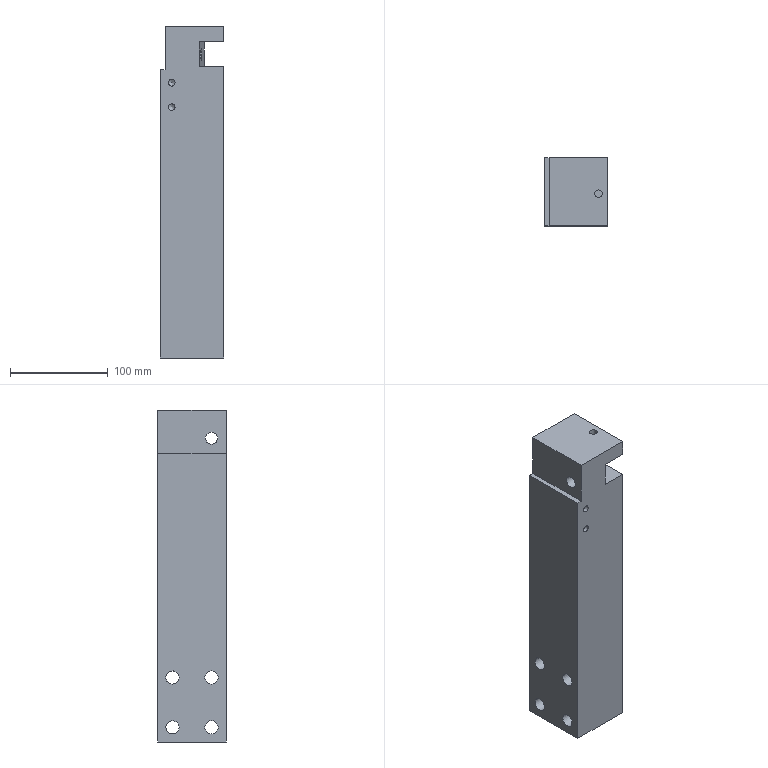Part | STEP file | lll_id3774_x_t | 1 solid | 34 faces | box 65 x 70 x 340 mm | volume 1424585 mm3 | plane 18 | cylinder 14 | cone 2 | commonest cylinder face diameters 13.509 x4 20.008 x4 6.806 x2 8 x2 12.5 x1 60 x1
STEP:
#1=CARTESIAN_POINT('',(3972.435,-498.677,125.));
#2=VERTEX_POINT('',#1);
#3=CARTESIAN_POINT('',(3972.435,-568.677,125.));
#4=VERTEX_POINT('',#3);
#5=CARTESIAN_POINT('',(3972.435,-533.677,125.));
#6=DIRECTION('',(0.,-1.,0.));
#7=VECTOR('',#6,1.);
#8=LINE('',#5,#7);
#9=EDGE_CURVE('',#2,#4,#8,.T.);
#10=ORIENTED_EDGE('',*,*,#9,.T.);
#11=CARTESIAN_POINT('',(3972.435,-568.677,170.));
#12=VERTEX_POINT('',#11);
#13=CARTESIAN_POINT('',(3972.435,-568.677,238.75));
#14=DIRECTION('',(0.,0.,1.));
#15=VECTOR('',#14,1.);
#16=LINE('',#13,#15);
#17=EDGE_CURVE('',#4,#12,#16,.T.);
#18=ORIENTED_EDGE('',*,*,#17,.T.);
#19=CARTESIAN_POINT('',(3972.435,-498.677,170.));
#20=VERTEX_POINT('',#19);
#21=CARTESIAN_POINT('',(3972.435,-530.677,170.));
#22=DIRECTION('',(0.,-1.,0.));
#23=VECTOR('',#22,1.);
#24=LINE('',#21,#23);
#25=EDGE_CURVE('',#20,#12,#24,.T.);
#26=ORIENTED_EDGE('',*,*,#25,.F.);
#27=CARTESIAN_POINT('',(3972.435,-498.677,238.75));
#28=DIRECTION('',(0.,0.,-1.));
#29=VECTOR('',#28,1.);
#30=LINE('',#27,#29);
#31=EDGE_CURVE('',#20,#2,#30,.T.);
#32=ORIENTED_EDGE('',*,*,#31,.T.);
#33=EDGE_LOOP('',(#10,#18,#26,#32));
#34=FACE_BOUND('',#33,.T.);
#35=CARTESIAN_POINT('',(3972.435,-547.427,141.25));
#36=VERTEX_POINT('',#35);
#37=CARTESIAN_POINT('',(3972.435,-553.677,141.25));
#38=DIRECTION('',(1.,0.,0.));
#39=DIRECTION('',(0.,1.,0.));
#40=AXIS2_PLACEMENT_3D('',#37,#38,#39);
#41=CIRCLE('',#40,6.25);
#42=EDGE_CURVE('',#36,#36,#41,.T.);
#43=ORIENTED_EDGE('',*,*,#42,.T.);
#44=EDGE_LOOP('',(#43));
#45=FACE_BOUND('',#44,.T.);
#46=CARTESIAN_POINT('',(3972.435,-533.677,0.));
#47=DIRECTION('',(-1.,0.,0.));
#48=DIRECTION('',(0.,0.,1.));
#49=AXIS2_PLACEMENT_3D('',#46,#47,#48);
#50=PLANE('',#49);
#51=ADVANCED_FACE('',(#34,#45),#50,.T.);
#52=CARTESIAN_POINT('',(4032.435,-568.677,-170.));
#53=VERTEX_POINT('',#52);
#54=CARTESIAN_POINT('',(3967.435,-568.677,-170.));
#55=VERTEX_POINT('',#54);
#56=CARTESIAN_POINT('',(4025.,-568.677,-170.));
#57=DIRECTION('',(-1.,0.,0.));
#58=VECTOR('',#57,1.);
#59=LINE('',#56,#58);
#60=EDGE_CURVE('',#53,#55,#59,.T.);
#61=ORIENTED_EDGE('',*,*,#60,.T.);
#62=CARTESIAN_POINT('',(3967.435,-498.677,-170.));
#63=VERTEX_POINT('',#62);
#64=CARTESIAN_POINT('',(3967.435,0.,-170.));
#65=DIRECTION('',(0.,1.,0.));
#66=VECTOR('',#65,1.);
#67=LINE('',#64,#66);
#68=EDGE_CURVE('',#55,#63,#67,.T.);
#69=ORIENTED_EDGE('',*,*,#68,.T.);
#70=CARTESIAN_POINT('',(4032.435,-498.677,-170.));
#71=VERTEX_POINT('',#70);
#72=CARTESIAN_POINT('',(3961.,-498.677,-170.));
#73=DIRECTION('',(1.,0.,0.));
#74=VECTOR('',#73,1.);
#75=LINE('',#72,#74);
#76=EDGE_CURVE('',#63,#71,#75,.T.);
#77=ORIENTED_EDGE('',*,*,#76,.T.);
#78=CARTESIAN_POINT('',(4032.435,0.,-170.));
#79=DIRECTION('',(0.,-1.,0.));
#80=VECTOR('',#79,1.);
#81=LINE('',#78,#80);
#82=EDGE_CURVE('',#71,#53,#81,.T.);
#83=ORIENTED_EDGE('',*,*,#82,.T.);
#84=EDGE_LOOP('',(#61,#69,#77,#83));
#85=FACE_OUTER_BOUND('',#84,.T.);
#86=CARTESIAN_POINT('',(2132.435,0.,-170.));
#87=DIRECTION('',(0.,0.,-1.));
#88=DIRECTION('',(-1.,0.,0.));
#89=AXIS2_PLACEMENT_3D('',#86,#87,#88);
#90=PLANE('',#89);
#91=ADVANCED_FACE('',(#85),#90,.T.);
#92=CARTESIAN_POINT('',(3975.804,-568.677,86.922));
#93=VERTEX_POINT('',#92);
#94=CARTESIAN_POINT('',(3979.207,-568.677,86.922));
#95=DIRECTION('',(0.,1.,0.));
#96=DIRECTION('',(-1.,0.,0.));
#97=AXIS2_PLACEMENT_3D('',#94,#95,#96);
#98=CIRCLE('',#97,3.403);
#99=EDGE_CURVE('',#93,#93,#98,.T.);
#100=ORIENTED_EDGE('',*,*,#99,.T.);
#101=EDGE_LOOP('',(#100));
#102=FACE_BOUND('',#101,.T.);
#103=CARTESIAN_POINT('',(3975.804,-568.677,111.922));
#104=VERTEX_POINT('',#103);
#105=CARTESIAN_POINT('',(3979.207,-568.677,111.922));
#106=DIRECTION('',(0.,1.,0.));
#107=DIRECTION('',(-1.,0.,0.));
#108=AXIS2_PLACEMENT_3D('',#105,#106,#107);
#109=CIRCLE('',#108,3.403);
#110=EDGE_CURVE('',#104,#104,#109,.T.);
#111=ORIENTED_EDGE('',*,*,#110,.T.);
#112=EDGE_LOOP('',(#111));
#113=FACE_BOUND('',#112,.T.);
#114=CARTESIAN_POINT('',(4032.435,-568.677,170.));
#115=VERTEX_POINT('',#114);
#116=CARTESIAN_POINT('',(3997.718,-568.677,170.));
#117=DIRECTION('',(-1.,0.,0.));
#118=VECTOR('',#117,1.);
#119=LINE('',#116,#118);
#120=EDGE_CURVE('',#115,#12,#119,.T.);
#121=ORIENTED_EDGE('',*,*,#120,.T.);
#122=ORIENTED_EDGE('',*,*,#17,.F.);
#123=CARTESIAN_POINT('',(3967.435,-568.677,125.));
#124=VERTEX_POINT('',#123);
#125=CARTESIAN_POINT('',(4002.435,-568.677,125.));
#126=DIRECTION('',(1.,0.,0.));
#127=VECTOR('',#126,1.);
#128=LINE('',#125,#127);
#129=EDGE_CURVE('',#124,#4,#128,.T.);
#130=ORIENTED_EDGE('',*,*,#129,.F.);
#131=CARTESIAN_POINT('',(3967.435,-568.677,238.75));
#132=DIRECTION('',(0.,0.,-1.));
#133=VECTOR('',#132,1.);
#134=LINE('',#131,#133);
#135=EDGE_CURVE('',#124,#55,#134,.T.);
#136=ORIENTED_EDGE('',*,*,#135,.T.);
#137=ORIENTED_EDGE('',*,*,#60,.F.);
#138=CARTESIAN_POINT('',(4032.435,-568.677,128.75));
#139=VERTEX_POINT('',#138);
#140=CARTESIAN_POINT('',(4032.435,-568.677,238.75));
#141=DIRECTION('',(0.,0.,-1.));
#142=VECTOR('',#141,1.);
#143=LINE('',#140,#142);
#144=EDGE_CURVE('',#139,#53,#143,.T.);
#145=ORIENTED_EDGE('',*,*,#144,.F.);
#146=CARTESIAN_POINT('',(4007.47,-568.677,128.75));
#147=VERTEX_POINT('',#146);
#148=CARTESIAN_POINT('',(4025.,-568.677,128.75));
#149=DIRECTION('',(-1.,0.,0.));
#150=VECTOR('',#149,1.);
#151=LINE('',#148,#150);
#152=EDGE_CURVE('',#139,#147,#151,.T.);
#153=ORIENTED_EDGE('',*,*,#152,.T.);
#154=CARTESIAN_POINT('',(4007.47,-568.677,153.75));
#155=VERTEX_POINT('',#154);
#156=CARTESIAN_POINT('',(4007.47,-568.677,238.75));
#157=DIRECTION('',(0.,0.,1.));
#158=VECTOR('',#157,1.);
#159=LINE('',#156,#158);
#160=EDGE_CURVE('',#147,#155,#159,.T.);
#161=ORIENTED_EDGE('',*,*,#160,.T.);
#162=CARTESIAN_POINT('',(4032.435,-568.677,153.75));
#163=VERTEX_POINT('',#162);
#164=CARTESIAN_POINT('',(4025.,-568.677,153.75));
#165=DIRECTION('',(-1.,0.,0.));
#166=VECTOR('',#165,1.);
#167=LINE('',#164,#166);
#168=EDGE_CURVE('',#163,#155,#167,.T.);
#169=ORIENTED_EDGE('',*,*,#168,.F.);
#170=CARTESIAN_POINT('',(4032.435,-568.677,238.75));
#171=DIRECTION('',(0.,0.,-1.));
#172=VECTOR('',#171,1.);
#173=LINE('',#170,#172);
#174=EDGE_CURVE('',#115,#163,#173,.T.);
#175=ORIENTED_EDGE('',*,*,#174,.F.);
#176=EDGE_LOOP('',(#121,#122,#130,#136,#137,#145,#153,#161,#169,#175));
#177=FACE_BOUND('',#176,.T.);
#178=CARTESIAN_POINT('',(4025.,-568.677,238.75));
#179=DIRECTION('',(0.,-1.,0.));
#180=DIRECTION('',(-1.,0.,0.));
#181=AXIS2_PLACEMENT_3D('',#178,#179,#180);
#182=PLANE('',#181);
#183=ADVANCED_FACE('',(#102,#113,#177),#182,.T.);
#184=ORIENTED_EDGE('',*,*,#76,.F.);
#185=CARTESIAN_POINT('',(3967.435,-498.677,125.));
#186=VERTEX_POINT('',#185);
#187=CARTESIAN_POINT('',(3967.435,-498.677,-60.));
#188=DIRECTION('',(0.,0.,-1.));
#189=VECTOR('',#188,1.);
#190=LINE('',#187,#189);
#191=EDGE_CURVE('',#186,#63,#190,.T.);
#192=ORIENTED_EDGE('',*,*,#191,.F.);
#193=CARTESIAN_POINT('',(3961.,-498.677,125.));
#194=DIRECTION('',(1.,0.,0.));
#195=VECTOR('',#194,1.);
#196=LINE('',#193,#195);
#197=EDGE_CURVE('',#186,#2,#196,.T.);
#198=ORIENTED_EDGE('',*,*,#197,.T.);
#199=ORIENTED_EDGE('',*,*,#31,.F.);
#200=CARTESIAN_POINT('',(4032.435,-498.677,170.));
#201=VERTEX_POINT('',#200);
#202=CARTESIAN_POINT('',(3961.,-498.677,170.));
#203=DIRECTION('',(-1.,0.,0.));
#204=VECTOR('',#203,1.);
#205=LINE('',#202,#204);
#206=EDGE_CURVE('',#201,#20,#205,.T.);
#207=ORIENTED_EDGE('',*,*,#206,.F.);
#208=CARTESIAN_POINT('',(4032.435,-498.677,153.75));
#209=VERTEX_POINT('',#208);
#210=CARTESIAN_POINT('',(4032.435,-498.677,238.75));
#211=DIRECTION('',(0.,0.,1.));
#212=VECTOR('',#211,1.);
#213=LINE('',#210,#212);
#214=EDGE_CURVE('',#209,#201,#213,.T.);
#215=ORIENTED_EDGE('',*,*,#214,.F.);
#216=CARTESIAN_POINT('',(4012.5,-498.677,153.75));
#217=VERTEX_POINT('',#216);
#218=CARTESIAN_POINT('',(3961.,-498.677,153.75));
#219=DIRECTION('',(1.,0.,0.));
#220=VECTOR('',#219,1.);
#221=LINE('',#218,#220);
#222=EDGE_CURVE('',#217,#209,#221,.T.);
#223=ORIENTED_EDGE('',*,*,#222,.F.);
#224=CARTESIAN_POINT('',(4012.5,-498.677,128.75));
#225=VERTEX_POINT('',#224);
#226=CARTESIAN_POINT('',(4012.5,-498.677,238.75));
#227=DIRECTION('',(0.,0.,1.));
#228=VECTOR('',#227,1.);
#229=LINE('',#226,#228);
#230=EDGE_CURVE('',#225,#217,#229,.T.);
#231=ORIENTED_EDGE('',*,*,#230,.F.);
#232=CARTESIAN_POINT('',(4032.435,-498.677,128.75));
#233=VERTEX_POINT('',#232);
#234=CARTESIAN_POINT('',(3961.,-498.677,128.75));
#235=DIRECTION('',(1.,0.,0.));
#236=VECTOR('',#235,1.);
#237=LINE('',#234,#236);
#238=EDGE_CURVE('',#225,#233,#237,.T.);
#239=ORIENTED_EDGE('',*,*,#238,.T.);
#240=CARTESIAN_POINT('',(4032.435,-498.677,238.75));
#241=DIRECTION('',(0.,0.,1.));
#242=VECTOR('',#241,1.);
#243=LINE('',#240,#242);
#244=EDGE_CURVE('',#71,#233,#243,.T.);
#245=ORIENTED_EDGE('',*,*,#244,.F.);
#246=EDGE_LOOP('',(#184,#192,#198,#199,#207,#215,#223,#231,#239,#245));
#247=FACE_OUTER_BOUND('',#246,.T.);
#248=CARTESIAN_POINT('',(3961.,-498.677,238.75));
#249=DIRECTION('',(0.,1.,0.));
#250=DIRECTION('',(0.,0.,-1.));
#251=AXIS2_PLACEMENT_3D('',#248,#249,#250);
#252=PLANE('',#251);
#253=ADVANCED_FACE('',(#247),#252,.T.);
#254=CARTESIAN_POINT('',(4019.,-535.677,170.));
#255=VERTEX_POINT('',#254);
#256=CARTESIAN_POINT('',(4023.,-535.677,170.));
#257=DIRECTION('',(0.,0.,-1.));
#258=DIRECTION('',(-1.,0.,0.));
#259=AXIS2_PLACEMENT_3D('',#256,#257,#258);
#260=CIRCLE('',#259,4.);
#261=EDGE_CURVE('',#255,#255,#260,.T.);
#262=ORIENTED_EDGE('',*,*,#261,.T.);
#263=EDGE_LOOP('',(#262));
#264=FACE_BOUND('',#263,.T.);
#265=ORIENTED_EDGE('',*,*,#25,.T.);
#266=ORIENTED_EDGE('',*,*,#120,.F.);
#267=CARTESIAN_POINT('',(4032.435,-530.677,170.));
#268=DIRECTION('',(0.,1.,0.));
#269=VECTOR('',#268,1.);
#270=LINE('',#267,#269);
#271=EDGE_CURVE('',#115,#201,#270,.T.);
#272=ORIENTED_EDGE('',*,*,#271,.T.);
#273=ORIENTED_EDGE('',*,*,#206,.T.);
#274=EDGE_LOOP('',(#265,#266,#272,#273));
#275=FACE_BOUND('',#274,.T.);
#276=CARTESIAN_POINT('',(3997.718,-530.677,170.));
#277=DIRECTION('',(0.,0.,-1.));
#278=DIRECTION('',(-1.,0.,0.));
#279=AXIS2_PLACEMENT_3D('',#276,#277,#278);
#280=PLANE('',#279);
#281=ADVANCED_FACE('',(#264,#275),#280,.F.);
#282=CARTESIAN_POINT('',(3997.435,-520.431,-155.));
#283=VERTEX_POINT('',#282);
#284=CARTESIAN_POINT('',(3997.435,-513.677,-155.));
#285=DIRECTION('',(1.,0.,0.));
#286=DIRECTION('',(0.,-1.,0.));
#287=AXIS2_PLACEMENT_3D('',#284,#285,#286);
#288=CIRCLE('',#287,6.755);
#289=EDGE_CURVE('',#283,#283,#288,.T.);
#290=ORIENTED_EDGE('',*,*,#289,.T.);
#291=EDGE_LOOP('',(#290));
#292=FACE_BOUND('',#291,.T.);
#293=CARTESIAN_POINT('',(3967.435,-513.677,-161.755));
#294=VERTEX_POINT('',#293);
#295=CARTESIAN_POINT('',(3967.435,-513.677,-155.));
#296=DIRECTION('',(-1.,0.,0.));
#297=DIRECTION('',(0.,0.,-1.));
#298=AXIS2_PLACEMENT_3D('',#295,#296,#297);
#299=CIRCLE('',#298,6.755);
#300=EDGE_CURVE('',#294,#294,#299,.T.);
#301=ORIENTED_EDGE('',*,*,#300,.T.);
#302=EDGE_LOOP('',(#301));
#303=FACE_BOUND('',#302,.T.);
#304=CARTESIAN_POINT('',(4032.435,-513.677,-155.));
#305=DIRECTION('',(-1.,0.,0.));
#306=DIRECTION('',(0.,0.,1.));
#307=AXIS2_PLACEMENT_3D('',#304,#305,#306);
#308=CYLINDRICAL_SURFACE('',#307,6.755);
#309=ADVANCED_FACE('',(#292,#303),#308,.F.);
#310=CARTESIAN_POINT('',(3997.435,-520.431,-104.));
#311=VERTEX_POINT('',#310);
#312=CARTESIAN_POINT('',(3997.435,-513.677,-104.));
#313=DIRECTION('',(1.,0.,0.));
#314=DIRECTION('',(0.,-1.,0.));
#315=AXIS2_PLACEMENT_3D('',#312,#313,#314);
#316=CIRCLE('',#315,6.755);
#317=EDGE_CURVE('',#311,#311,#316,.T.);
#318=ORIENTED_EDGE('',*,*,#317,.T.);
#319=EDGE_LOOP('',(#318));
#320=FACE_BOUND('',#319,.T.);
#321=CARTESIAN_POINT('',(3967.435,-513.677,-110.754));
#322=VERTEX_POINT('',#321);
#323=CARTESIAN_POINT('',(3967.435,-513.677,-104.));
#324=DIRECTION('',(-1.,0.,0.));
#325=DIRECTION('',(0.,0.,-1.));
#326=AXIS2_PLACEMENT_3D('',#323,#324,#325);
#327=CIRCLE('',#326,6.755);
#328=EDGE_CURVE('',#322,#322,#327,.T.);
#329=ORIENTED_EDGE('',*,*,#328,.T.);
#330=EDGE_LOOP('',(#329));
#331=FACE_BOUND('',#330,.T.);
#332=CARTESIAN_POINT('',(4032.435,-513.677,-104.));
#333=DIRECTION('',(-1.,0.,0.));
#334=DIRECTION('',(0.,0.,1.));
#335=AXIS2_PLACEMENT_3D('',#332,#333,#334);
#336=CYLINDRICAL_SURFACE('',#335,6.755);
#337=ADVANCED_FACE('',(#320,#331),#336,.F.);
#338=CARTESIAN_POINT('',(3997.435,-553.677,-97.246));
#339=VERTEX_POINT('',#338);
#340=CARTESIAN_POINT('',(3997.435,-553.677,-104.));
#341=DIRECTION('',(-1.,0.,0.));
#342=DIRECTION('',(0.,0.,1.));
#343=AXIS2_PLACEMENT_3D('',#340,#341,#342);
#344=CIRCLE('',#343,6.755);
#345=EDGE_CURVE('',#339,#339,#344,.T.);
#346=ORIENTED_EDGE('',*,*,#345,.F.);
#347=EDGE_LOOP('',(#346));
#348=FACE_BOUND('',#347,.T.);
#349=CARTESIAN_POINT('',(3967.435,-553.677,-110.754));
#350=VERTEX_POINT('',#349);
#351=CARTESIAN_POINT('',(3967.435,-553.677,-104.));
#352=DIRECTION('',(-1.,0.,0.));
#353=DIRECTION('',(0.,0.,-1.));
#354=AXIS2_PLACEMENT_3D('',#351,#352,#353);
#355=CIRCLE('',#354,6.755);
#356=EDGE_CURVE('',#350,#350,#355,.T.);
#357=ORIENTED_EDGE('',*,*,#356,.T.);
#358=EDGE_LOOP('',(#357));
#359=FACE_BOUND('',#358,.T.);
#360=CARTESIAN_POINT('',(4032.435,-553.677,-104.));
#361=DIRECTION('',(-1.,0.,0.));
#362=DIRECTION('',(0.,0.,1.));
#363=AXIS2_PLACEMENT_3D('',#360,#361,#362);
#364=CYLINDRICAL_SURFACE('',#363,6.755);
#365=ADVANCED_FACE('',(#348,#359),#364,.F.);
#366=CARTESIAN_POINT('',(3997.435,-553.677,-148.245));
#367=VERTEX_POINT('',#366);
#368=CARTESIAN_POINT('',(3997.435,-553.677,-155.));
#369=DIRECTION('',(-1.,0.,0.));
#370=DIRECTION('',(0.,0.,1.));
#371=AXIS2_PLACEMENT_3D('',#368,#369,#370);
#372=CIRCLE('',#371,6.755);
#373=EDGE_CURVE('',#367,#367,#372,.T.);
#374=ORIENTED_EDGE('',*,*,#373,.F.);
#375=EDGE_LOOP('',(#374));
#376=FACE_BOUND('',#375,.T.);
#377=CARTESIAN_POINT('',(3967.435,-553.677,-161.755));
#378=VERTEX_POINT('',#377);
#379=CARTESIAN_POINT('',(3967.435,-553.677,-155.));
#380=DIRECTION('',(-1.,0.,0.));
#381=DIRECTION('',(0.,0.,-1.));
#382=AXIS2_PLACEMENT_3D('',#379,#380,#381);
#383=CIRCLE('',#382,6.755);
#384=EDGE_CURVE('',#378,#378,#383,.T.);
#385=ORIENTED_EDGE('',*,*,#384,.T.);
#386=EDGE_LOOP('',(#385));
#387=FACE_BOUND('',#386,.T.);
#388=CARTESIAN_POINT('',(4032.435,-553.677,-155.));
#389=DIRECTION('',(-1.,0.,0.));
#390=DIRECTION('',(0.,0.,1.));
#391=AXIS2_PLACEMENT_3D('',#388,#389,#390);
#392=CYLINDRICAL_SURFACE('',#391,6.755);
#393=ADVANCED_FACE('',(#376,#387),#392,.F.);
#394=CARTESIAN_POINT('',(4032.435,-553.677,-144.996));
#395=VERTEX_POINT('',#394);
#396=CARTESIAN_POINT('',(4032.435,-553.677,-155.));
#397=DIRECTION('',(-1.,0.,0.));
#398=DIRECTION('',(0.,0.,1.));
#399=AXIS2_PLACEMENT_3D('',#396,#397,#398);
#400=CIRCLE('',#399,10.004);
#401=EDGE_CURVE('',#395,#395,#400,.T.);
#402=ORIENTED_EDGE('',*,*,#401,.T.);
#403=EDGE_LOOP('',(#402));
#404=FACE_BOUND('',#403,.T.);
#405=CARTESIAN_POINT('',(4032.435,-553.677,-93.996));
#406=VERTEX_POINT('',#405);
#407=CARTESIAN_POINT('',(4032.435,-553.677,-104.));
#408=DIRECTION('',(-1.,0.,0.));
#409=DIRECTION('',(0.,0.,1.));
#410=AXIS2_PLACEMENT_3D('',#407,#408,#409);
#411=CIRCLE('',#410,10.004);
#412=EDGE_CURVE('',#406,#406,#411,.T.);
#413=ORIENTED_EDGE('',*,*,#412,.T.);
#414=EDGE_LOOP('',(#413));
#415=FACE_BOUND('',#414,.T.);
#416=CARTESIAN_POINT('',(4032.435,-513.677,-144.996));
#417=VERTEX_POINT('',#416);
#418=CARTESIAN_POINT('',(4032.435,-513.677,-155.));
#419=DIRECTION('',(1.,0.,0.));
#420=DIRECTION('',(0.,0.,1.));
#421=AXIS2_PLACEMENT_3D('',#418,#419,#420);
#422=CIRCLE('',#421,10.004);
#423=EDGE_CURVE('',#417,#417,#422,.T.);
#424=ORIENTED_EDGE('',*,*,#423,.F.);
#425=EDGE_LOOP('',(#424));
#426=FACE_BOUND('',#425,.T.);
#427=ORIENTED_EDGE('',*,*,#144,.T.);
#428=ORIENTED_EDGE('',*,*,#82,.F.);
#429=ORIENTED_EDGE('',*,*,#244,.T.);
#430=CARTESIAN_POINT('',(4032.435,-271.677,128.75));
#431=DIRECTION('',(0.,-1.,0.));
#432=VECTOR('',#431,1.);
#433=LINE('',#430,#432);
#434=EDGE_CURVE('',#233,#139,#433,.T.);
#435=ORIENTED_EDGE('',*,*,#434,.T.);
#436=EDGE_LOOP('',(#427,#428,#429,#435));
#437=FACE_BOUND('',#436,.T.);
#438=CARTESIAN_POINT('',(4032.435,-513.677,-93.996));
#439=VERTEX_POINT('',#438);
#440=CARTESIAN_POINT('',(4032.435,-513.677,-104.));
#441=DIRECTION('',(1.,0.,0.));
#442=DIRECTION('',(0.,0.,1.));
#443=AXIS2_PLACEMENT_3D('',#440,#441,#442);
#444=CIRCLE('',#443,10.004);
#445=EDGE_CURVE('',#439,#439,#444,.T.);
#446=ORIENTED_EDGE('',*,*,#445,.F.);
#447=EDGE_LOOP('',(#446));
#448=FACE_BOUND('',#447,.T.);
#449=CARTESIAN_POINT('',(4032.435,-533.177,50.));
#450=DIRECTION('',(-1.,0.,0.));
#451=DIRECTION('',(0.,0.,1.));
#452=AXIS2_PLACEMENT_3D('',#449,#450,#451);
#453=PLANE('',#452);
#454=ADVANCED_FACE('',(#404,#415,#426,#437,#448),#453,.F.);
#455=CARTESIAN_POINT('',(4012.319,-524.673,153.75));
#456=VERTEX_POINT('',#455);
#457=CARTESIAN_POINT('',(4012.5,-521.386,153.75));
#458=VERTEX_POINT('',#457);
#459=CARTESIAN_POINT('',(3982.5,-521.386,153.75));
#460=DIRECTION('',(0.,0.,1.));
#461=DIRECTION('',(1.,0.,0.));
#462=AXIS2_PLACEMENT_3D('',#459,#460,#461);
#463=CIRCLE('',#462,30.);
#464=EDGE_CURVE('',#456,#458,#463,.T.);
#465=ORIENTED_EDGE('',*,*,#464,.F.);
#466=CARTESIAN_POINT('',(4012.319,-524.673,128.75));
#467=VERTEX_POINT('',#466);
#468=CARTESIAN_POINT('',(4012.319,-524.673,128.75));
#469=DIRECTION('',(0.,0.,1.));
#470=VECTOR('',#469,1.);
#471=LINE('',#468,#470);
#472=EDGE_CURVE('',#467,#456,#471,.T.);
#473=ORIENTED_EDGE('',*,*,#472,.F.);
#474=CARTESIAN_POINT('',(4012.5,-521.386,128.75));
#475=VERTEX_POINT('',#474);
#476=CARTESIAN_POINT('',(3982.5,-521.386,128.75));
#477=DIRECTION('',(0.,0.,-1.));
#478=DIRECTION('',(1.,0.,0.));
#479=AXIS2_PLACEMENT_3D('',#476,#477,#478);
#480=CIRCLE('',#479,30.);
#481=EDGE_CURVE('',#475,#467,#480,.T.);
#482=ORIENTED_EDGE('',*,*,#481,.F.);
#483=CARTESIAN_POINT('',(4012.5,-521.386,128.75));
#484=DIRECTION('',(0.,0.,-1.));
#485=VECTOR('',#484,1.);
#486=LINE('',#483,#485);
#487=EDGE_CURVE('',#458,#475,#486,.T.);
#488=ORIENTED_EDGE('',*,*,#487,.F.);
#489=EDGE_LOOP('',(#465,#473,#482,#488));
#490=FACE_OUTER_BOUND('',#489,.T.);
#491=CARTESIAN_POINT('',(3982.5,-521.386,128.75));
#492=DIRECTION('',(0.,0.,1.));
#493=DIRECTION('',(-1.,0.,0.));
#494=AXIS2_PLACEMENT_3D('',#491,#492,#493);
#495=CYLINDRICAL_SURFACE('',#494,30.);
#496=ADVANCED_FACE('',(#490),#495,.T.);
#497=CARTESIAN_POINT('',(4009.812,-547.427,141.25));
#498=VERTEX_POINT('',#497);
#499=CARTESIAN_POINT('',(4009.123,-553.677,141.25));
#500=DIRECTION('',(0.994,-0.1095,0.));
#501=DIRECTION('',(0.1095,0.994,0.));
#502=AXIS2_PLACEMENT_3D('',#499,#500,#501);
#503=ELLIPSE('',#502,6.288,6.25);
#504=EDGE_CURVE('',#498,#498,#503,.T.);
#505=ORIENTED_EDGE('',*,*,#504,.F.);
#506=EDGE_LOOP('',(#505));
#507=FACE_BOUND('',#506,.T.);
#508=CARTESIAN_POINT('',(4032.949,-337.487,128.75));
#509=DIRECTION('',(-0.1095,-0.994,0.));
#510=VECTOR('',#509,1.);
#511=LINE('',#508,#510);
#512=EDGE_CURVE('',#467,#147,#511,.T.);
#513=ORIENTED_EDGE('',*,*,#512,.F.);
#514=ORIENTED_EDGE('',*,*,#472,.T.);
#515=CARTESIAN_POINT('',(4012.539,-522.68,153.75));
#516=DIRECTION('',(0.1095,0.994,0.));
#517=VECTOR('',#516,1.);
#518=LINE('',#515,#517);
#519=EDGE_CURVE('',#155,#456,#518,.T.);
#520=ORIENTED_EDGE('',*,*,#519,.F.);
#521=ORIENTED_EDGE('',*,*,#160,.F.);
#522=EDGE_LOOP('',(#513,#514,#520,#521));
#523=FACE_BOUND('',#522,.T.);
#524=CARTESIAN_POINT('',(4012.539,-522.68,128.75));
#525=DIRECTION('',(0.994,-0.1095,0.));
#526=DIRECTION('',(0.,0.,-1.));
#527=AXIS2_PLACEMENT_3D('',#524,#525,#526);
#528=PLANE('',#527);
#529=ADVANCED_FACE('',(#507,#523),#528,.T.);
#530=ORIENTED_EDGE('',*,*,#434,.F.);
#531=ORIENTED_EDGE('',*,*,#238,.F.);
#532=CARTESIAN_POINT('',(4012.5,-377.103,128.75));
#533=DIRECTION('',(0.,-1.,0.));
#534=VECTOR('',#533,1.);
#535=LINE('',#532,#534);
#536=EDGE_CURVE('',#225,#475,#535,.T.);
#537=ORIENTED_EDGE('',*,*,#536,.T.);
#538=ORIENTED_EDGE('',*,*,#481,.T.);
#539=ORIENTED_EDGE('',*,*,#512,.T.);
#540=ORIENTED_EDGE('',*,*,#152,.F.);
#541=EDGE_LOOP('',(#530,#531,#537,#538,#539,#540));
#542=FACE_BOUND('',#541,.T.);
#543=CARTESIAN_POINT('',(4027.,-535.677,128.75));
#544=VERTEX_POINT('',#543);
#545=CARTESIAN_POINT('',(4023.,-535.677,128.75));
#546=DIRECTION('',(0.,0.,1.));
#547=DIRECTION('',(1.,0.,0.));
#548=AXIS2_PLACEMENT_3D('',#545,#546,#547);
#549=CIRCLE('',#548,4.);
#550=EDGE_CURVE('',#544,#544,#549,.T.);
#551=ORIENTED_EDGE('',*,*,#550,.F.);
#552=EDGE_LOOP('',(#551));
#553=FACE_BOUND('',#552,.T.);
#554=CARTESIAN_POINT('',(3157.,-271.677,128.75));
#555=DIRECTION('',(0.,0.,1.));
#556=DIRECTION('',(-1.,0.,0.));
#557=AXIS2_PLACEMENT_3D('',#554,#555,#556);
#558=PLANE('',#557);
#559=ADVANCED_FACE('',(#542,#553),#558,.T.);
#560=CARTESIAN_POINT('',(4012.5,-377.103,153.75));
#561=DIRECTION('',(0.,1.,0.));
#562=VECTOR('',#561,1.);
#563=LINE('',#560,#562);
#564=EDGE_CURVE('',#458,#217,#563,.T.);
#565=ORIENTED_EDGE('',*,*,#564,.F.);
#566=ORIENTED_EDGE('',*,*,#487,.T.);
#567=ORIENTED_EDGE('',*,*,#536,.F.);
#568=ORIENTED_EDGE('',*,*,#230,.T.);
#569=EDGE_LOOP('',(#565,#566,#567,#568));
#570=FACE_OUTER_BOUND('',#569,.T.);
#571=CARTESIAN_POINT('',(4012.5,-377.103,128.75));
#572=DIRECTION('',(-1.,0.,0.));
#573=DIRECTION('',(0.,0.,-1.));
#574=AXIS2_PLACEMENT_3D('',#571,#572,#573);
#575=PLANE('',#574);
#576=ADVANCED_FACE('',(#570),#575,.F.);
#577=CARTESIAN_POINT('',(4027.,-535.677,153.75));
#578=VERTEX_POINT('',#577);
#579=CARTESIAN_POINT('',(4023.,-535.677,153.75));
#580=DIRECTION('',(0.,0.,-1.));
#581=DIRECTION('',(1.,0.,0.));
#582=AXIS2_PLACEMENT_3D('',#579,#580,#581);
#583=CIRCLE('',#582,4.);
#584=EDGE_CURVE('',#578,#578,#583,.T.);
#585=ORIENTED_EDGE('',*,*,#584,.F.);
#586=EDGE_LOOP('',(#585));
#587=FACE_BOUND('',#586,.T.);
#588=ORIENTED_EDGE('',*,*,#222,.T.);
#589=CARTESIAN_POINT('',(4032.435,-377.103,153.75));
#590=DIRECTION('',(0.,-1.,0.));
#591=VECTOR('',#590,1.);
#592=LINE('',#589,#591);
#593=EDGE_CURVE('',#209,#163,#592,.T.);
#594=ORIENTED_EDGE('',*,*,#593,.T.);
#595=ORIENTED_EDGE('',*,*,#168,.T.);
#596=ORIENTED_EDGE('',*,*,#519,.T.);
#597=ORIENTED_EDGE('',*,*,#464,.T.);
#598=ORIENTED_EDGE('',*,*,#564,.T.);
#599=EDGE_LOOP('',(#588,#594,#595,#596,#597,#598));
#600=FACE_BOUND('',#599,.T.);
#601=CARTESIAN_POINT('',(4015.5,-377.103,153.75));
#602=DIRECTION('',(0.,0.,1.));
#603=DIRECTION('',(-1.,0.,0.));
#604=AXIS2_PLACEMENT_3D('',#601,#602,#603);
#605=PLANE('',#604);
#606=ADVANCED_FACE('',(#587,#600),#605,.F.);
#607=ORIENTED_EDGE('',*,*,#261,.F.);
#608=EDGE_LOOP('',(#607));
#609=FACE_BOUND('',#608,.T.);
#610=ORIENTED_EDGE('',*,*,#584,.T.);
#611=EDGE_LOOP('',(#610));
#612=FACE_BOUND('',#611,.T.);
#613=CARTESIAN_POINT('',(4023.,-535.677,118.75));
#614=DIRECTION('',(0.,0.,1.));
#615=DIRECTION('',(-1.,0.,0.));
#616=AXIS2_PLACEMENT_3D('',#613,#614,#615);
#617=CYLINDRICAL_SURFACE('',#616,4.);
#618=ADVANCED_FACE('',(#609,#612),#617,.F.);
#619=ORIENTED_EDGE('',*,*,#550,.T.);
#620=EDGE_LOOP('',(#619));
#621=FACE_BOUND('',#620,.T.);
#622=CARTESIAN_POINT('',(4019.,-535.677,118.75));
#623=VERTEX_POINT('',#622);
#624=CARTESIAN_POINT('',(4023.,-535.677,118.75));
#625=DIRECTION('',(0.,0.,-1.));
#626=DIRECTION('',(-1.,0.,0.));
#627=AXIS2_PLACEMENT_3D('',#624,#625,#626);
#628=CIRCLE('',#627,4.);
#629=EDGE_CURVE('',#623,#623,#628,.T.);
#630=ORIENTED_EDGE('',*,*,#629,.T.);
#631=EDGE_LOOP('',(#630));
#632=FACE_BOUND('',#631,.T.);
#633=CARTESIAN_POINT('',(4023.,-535.677,169.75));
#634=DIRECTION('',(0.,0.,-1.));
#635=DIRECTION('',(-1.,0.,0.));
#636=AXIS2_PLACEMENT_3D('',#633,#634,#635);
#637=CYLINDRICAL_SURFACE('',#636,4.);
#638=ADVANCED_FACE('',(#621,#632),#637,.F.);
#639=ORIENTED_EDGE('',*,*,#629,.F.);
#640=EDGE_LOOP('',(#639));
#641=FACE_OUTER_BOUND('',#640,.T.);
#642=CARTESIAN_POINT('',(4023.,-535.677,118.75));
#643=DIRECTION('',(0.,0.,-1.));
#644=DIRECTION('',(1.,0.,0.));
#645=AXIS2_PLACEMENT_3D('',#642,#643,#644);
#646=PLANE('',#645);
#647=ADVANCED_FACE('',(#641),#646,.F.);
#648=ORIENTED_EDGE('',*,*,#214,.T.);
#649=ORIENTED_EDGE('',*,*,#271,.F.);
#650=ORIENTED_EDGE('',*,*,#174,.T.);
#651=ORIENTED_EDGE('',*,*,#593,.F.);
#652=EDGE_LOOP('',(#648,#649,#650,#651));
#653=FACE_OUTER_BOUND('',#652,.T.);
#654=CARTESIAN_POINT('',(4032.435,-533.177,50.));
#655=DIRECTION('',(-1.,0.,0.));
#656=DIRECTION('',(0.,0.,1.));
#657=AXIS2_PLACEMENT_3D('',#654,#655,#656);
#658=PLANE('',#657);
#659=ADVANCED_FACE('',(#653),#658,.F.);
#660=ORIENTED_EDGE('',*,*,#289,.F.);
#661=EDGE_LOOP('',(#660));
#662=FACE_BOUND('',#661,.T.);
#663=CARTESIAN_POINT('',(3997.435,-523.681,-155.));
#664=VERTEX_POINT('',#663);
#665=CARTESIAN_POINT('',(3997.435,-513.677,-155.));
#666=DIRECTION('',(1.,0.,0.));
#667=DIRECTION('',(0.,-1.,0.));
#668=AXIS2_PLACEMENT_3D('',#665,#666,#667);
#669=CIRCLE('',#668,10.004);
#670=EDGE_CURVE('',#664,#664,#669,.T.);
#671=ORIENTED_EDGE('',*,*,#670,.T.);
#672=EDGE_LOOP('',(#671));
#673=FACE_BOUND('',#672,.T.);
#674=CARTESIAN_POINT('',(3997.435,-513.677,-155.));
#675=DIRECTION('',(-1.,0.,0.));
#676=DIRECTION('',(0.,0.,1.));
#677=AXIS2_PLACEMENT_3D('',#674,#675,#676);
#678=PLANE('',#677);
#679=ADVANCED_FACE('',(#662,#673),#678,.F.);
#680=ORIENTED_EDGE('',*,*,#670,.F.);
#681=EDGE_LOOP('',(#680));
#682=FACE_BOUND('',#681,.T.);
#683=ORIENTED_EDGE('',*,*,#423,.T.);
#684=EDGE_LOOP('',(#683));
#685=FACE_BOUND('',#684,.T.);
#686=CARTESIAN_POINT('',(4032.435,-513.677,-155.));
#687=DIRECTION('',(-1.,0.,0.));
#688=DIRECTION('',(0.,0.,1.));
#689=AXIS2_PLACEMENT_3D('',#686,#687,#688);
#690=CYLINDRICAL_SURFACE('',#689,10.004);
#691=ADVANCED_FACE('',(#682,#685),#690,.F.);
#692=ORIENTED_EDGE('',*,*,#317,.F.);
#693=EDGE_LOOP('',(#692));
#694=FACE_BOUND('',#693,.T.);
#695=CARTESIAN_POINT('',(3997.435,-523.681,-104.));
#696=VERTEX_POINT('',#695);
#697=CARTESIAN_POINT('',(3997.435,-513.677,-104.));
#698=DIRECTION('',(1.,0.,0.));
#699=DIRECTION('',(0.,-1.,0.));
#700=AXIS2_PLACEMENT_3D('',#697,#698,#699);
#701=CIRCLE('',#700,10.004);
#702=EDGE_CURVE('',#696,#696,#701,.T.);
#703=ORIENTED_EDGE('',*,*,#702,.T.);
#704=EDGE_LOOP('',(#703));
#705=FACE_BOUND('',#704,.T.);
#706=CARTESIAN_POINT('',(3997.435,-513.677,-104.));
#707=DIRECTION('',(-1.,0.,0.));
#708=DIRECTION('',(0.,0.,1.));
#709=AXIS2_PLACEMENT_3D('',#706,#707,#708);
#710=PLANE('',#709);
#711=ADVANCED_FACE('',(#694,#705),#710,.F.);
#712=ORIENTED_EDGE('',*,*,#702,.F.);
#713=EDGE_LOOP('',(#712));
#714=FACE_BOUND('',#713,.T.);
#715=ORIENTED_EDGE('',*,*,#445,.T.);
#716=EDGE_LOOP('',(#715));
#717=FACE_BOUND('',#716,.T.);
#718=CARTESIAN_POINT('',(4032.435,-513.677,-104.));
#719=DIRECTION('',(-1.,0.,0.));
#720=DIRECTION('',(0.,0.,1.));
#721=AXIS2_PLACEMENT_3D('',#718,#719,#720);
#722=CYLINDRICAL_SURFACE('',#721,10.004);
#723=ADVANCED_FACE('',(#714,#717),#722,.F.);
#724=ORIENTED_EDGE('',*,*,#345,.T.);
#725=EDGE_LOOP('',(#724));
#726=FACE_BOUND('',#725,.T.);
#727=CARTESIAN_POINT('',(3997.435,-553.677,-93.996));
#728=VERTEX_POINT('',#727);
#729=CARTESIAN_POINT('',(3997.435,-553.677,-104.));
#730=DIRECTION('',(-1.,0.,0.));
#731=DIRECTION('',(0.,0.,1.));
#732=AXIS2_PLACEMENT_3D('',#729,#730,#731);
#733=CIRCLE('',#732,10.004);
#734=EDGE_CURVE('',#728,#728,#733,.T.);
#735=ORIENTED_EDGE('',*,*,#734,.F.);
#736=EDGE_LOOP('',(#735));
#737=FACE_BOUND('',#736,.T.);
#738=CARTESIAN_POINT('',(3997.435,-553.677,-104.));
#739=DIRECTION('',(-1.,0.,0.));
#740=DIRECTION('',(0.,0.,1.));
#741=AXIS2_PLACEMENT_3D('',#738,#739,#740);
#742=PLANE('',#741);
#743=ADVANCED_FACE('',(#726,#737),#742,.F.);
#744=ORIENTED_EDGE('',*,*,#734,.T.);
#745=EDGE_LOOP('',(#744));
#746=FACE_BOUND('',#745,.T.);
#747=ORIENTED_EDGE('',*,*,#412,.F.);
#748=EDGE_LOOP('',(#747));
#749=FACE_BOUND('',#748,.T.);
#750=CARTESIAN_POINT('',(4032.435,-553.677,-104.));
#751=DIRECTION('',(-1.,0.,0.));
#752=DIRECTION('',(0.,0.,1.));
#753=AXIS2_PLACEMENT_3D('',#750,#751,#752);
#754=CYLINDRICAL_SURFACE('',#753,10.004);
#755=ADVANCED_FACE('',(#746,#749),#754,.F.);
#756=ORIENTED_EDGE('',*,*,#373,.T.);
#757=EDGE_LOOP('',(#756));
#758=FACE_BOUND('',#757,.T.);
#759=CARTESIAN_POINT('',(3997.435,-553.677,-144.996));
#760=VERTEX_POINT('',#759);
#761=CARTESIAN_POINT('',(3997.435,-553.677,-155.));
#762=DIRECTION('',(-1.,0.,0.));
#763=DIRECTION('',(0.,0.,1.));
#764=AXIS2_PLACEMENT_3D('',#761,#762,#763);
#765=CIRCLE('',#764,10.004);
#766=EDGE_CURVE('',#760,#760,#765,.T.);
#767=ORIENTED_EDGE('',*,*,#766,.F.);
#768=EDGE_LOOP('',(#767));
#769=FACE_BOUND('',#768,.T.);
#770=CARTESIAN_POINT('',(3997.435,-553.677,-155.));
#771=DIRECTION('',(-1.,0.,0.));
#772=DIRECTION('',(0.,0.,1.));
#773=AXIS2_PLACEMENT_3D('',#770,#771,#772);
#774=PLANE('',#773);
#775=ADVANCED_FACE('',(#758,#769),#774,.F.);
#776=ORIENTED_EDGE('',*,*,#766,.T.);
#777=EDGE_LOOP('',(#776));
#778=FACE_BOUND('',#777,.T.);
#779=ORIENTED_EDGE('',*,*,#401,.F.);
#780=EDGE_LOOP('',(#779));
#781=FACE_BOUND('',#780,.T.);
#782=CARTESIAN_POINT('',(4032.435,-553.677,-155.));
#783=DIRECTION('',(-1.,0.,0.));
#784=DIRECTION('',(0.,0.,1.));
#785=AXIS2_PLACEMENT_3D('',#782,#783,#784);
#786=CYLINDRICAL_SURFACE('',#785,10.004);
#787=ADVANCED_FACE('',(#778,#781),#786,.F.);
#788=ORIENTED_EDGE('',*,*,#300,.F.);
#789=EDGE_LOOP('',(#788));
#790=FACE_BOUND('',#789,.T.);
#791=ORIENTED_EDGE('',*,*,#328,.F.);
#792=EDGE_LOOP('',(#791));
#793=FACE_BOUND('',#792,.T.);
#794=ORIENTED_EDGE('',*,*,#356,.F.);
#795=EDGE_LOOP('',(#794));
#796=FACE_BOUND('',#795,.T.);
#797=ORIENTED_EDGE('',*,*,#384,.F.);
#798=EDGE_LOOP('',(#797));
#799=FACE_BOUND('',#798,.T.);
#800=ORIENTED_EDGE('',*,*,#135,.F.);
#801=CARTESIAN_POINT('',(3967.435,-533.677,125.));
#802=DIRECTION('',(0.,1.,0.));
#803=VECTOR('',#802,1.);
#804=LINE('',#801,#803);
#805=EDGE_CURVE('',#124,#186,#804,.T.);
#806=ORIENTED_EDGE('',*,*,#805,.T.);
#807=ORIENTED_EDGE('',*,*,#191,.T.);
#808=ORIENTED_EDGE('',*,*,#68,.F.);
#809=EDGE_LOOP('',(#800,#806,#807,#808));
#810=FACE_BOUND('',#809,.T.);
#811=CARTESIAN_POINT('',(3967.435,0.,-60.));
#812=DIRECTION('',(1.,0.,0.));
#813=DIRECTION('',(0.,0.,-1.));
#814=AXIS2_PLACEMENT_3D('',#811,#812,#813);
#815=PLANE('',#814);
#816=ADVANCED_FACE('',(#790,#793,#796,#799,#810),#815,.F.);
#817=ORIENTED_EDGE('',*,*,#805,.F.);
#818=ORIENTED_EDGE('',*,*,#129,.T.);
#819=ORIENTED_EDGE('',*,*,#9,.F.);
#820=ORIENTED_EDGE('',*,*,#197,.F.);
#821=EDGE_LOOP('',(#817,#818,#819,#820));
#822=FACE_OUTER_BOUND('',#821,.T.);
#823=CARTESIAN_POINT('',(4002.435,-533.677,125.));
#824=DIRECTION('',(0.,0.,1.));
#825=DIRECTION('',(1.,0.,0.));
#826=AXIS2_PLACEMENT_3D('',#823,#824,#825);
#827=PLANE('',#826);
#828=ADVANCED_FACE('',(#822),#827,.T.);
#829=ORIENTED_EDGE('',*,*,#42,.F.);
#830=EDGE_LOOP('',(#829));
#831=FACE_BOUND('',#830,.T.);
#832=ORIENTED_EDGE('',*,*,#504,.T.);
#833=EDGE_LOOP('',(#832));
#834=FACE_BOUND('',#833,.T.);
#835=CARTESIAN_POINT('',(3972.435,-553.677,141.25));
#836=DIRECTION('',(1.,0.,0.));
#837=DIRECTION('',(0.,-1.,0.));
#838=AXIS2_PLACEMENT_3D('',#835,#836,#837);
#839=CYLINDRICAL_SURFACE('',#838,6.25);
#840=ADVANCED_FACE('',(#831,#834),#839,.F.);
#841=CARTESIAN_POINT('',(3975.804,-543.677,111.922));
#842=VERTEX_POINT('',#841);
#843=CARTESIAN_POINT('',(3979.207,-543.677,111.922));
#844=DIRECTION('',(0.,-1.,0.));
#845=DIRECTION('',(-1.,0.,0.));
#846=AXIS2_PLACEMENT_3D('',#843,#844,#845);
#847=CIRCLE('',#846,3.403);
#848=EDGE_CURVE('',#842,#842,#847,.T.);
#849=ORIENTED_EDGE('',*,*,#848,.T.);
#850=EDGE_LOOP('',(#849));
#851=FACE_BOUND('',#850,.T.);
#852=CARTESIAN_POINT('',(3979.207,-541.632,111.922));
#853=VERTEX_POINT('',#852);
#854=VERTEX_LOOP('',#853);
#855=FACE_BOUND('',#854,.T.);
#856=CARTESIAN_POINT('',(3979.207,-543.677,111.922));
#857=DIRECTION('',(0.,-1.,0.));
#858=DIRECTION('',(-1.,0.,0.));
#859=AXIS2_PLACEMENT_3D('',#856,#857,#858);
#860=CONICAL_SURFACE('',#859,3.403,59.);
#861=ADVANCED_FACE('',(#851,#855),#860,.F.);
#862=ORIENTED_EDGE('',*,*,#848,.F.);
#863=EDGE_LOOP('',(#862));
#864=FACE_BOUND('',#863,.T.);
#865=ORIENTED_EDGE('',*,*,#110,.F.);
#866=EDGE_LOOP('',(#865));
#867=FACE_BOUND('',#866,.T.);
#868=CARTESIAN_POINT('',(3979.207,-568.677,111.922));
#869=DIRECTION('',(0.,1.,0.));
#870=DIRECTION('',(1.,0.,0.));
#871=AXIS2_PLACEMENT_3D('',#868,#869,#870);
#872=CYLINDRICAL_SURFACE('',#871,3.403);
#873=ADVANCED_FACE('',(#864,#867),#872,.F.);
#874=CARTESIAN_POINT('',(3975.804,-543.677,86.922));
#875=VERTEX_POINT('',#874);
#876=CARTESIAN_POINT('',(3979.207,-543.677,86.922));
#877=DIRECTION('',(0.,-1.,0.));
#878=DIRECTION('',(-1.,0.,0.));
#879=AXIS2_PLACEMENT_3D('',#876,#877,#878);
#880=CIRCLE('',#879,3.403);
#881=EDGE_CURVE('',#875,#875,#880,.T.);
#882=ORIENTED_EDGE('',*,*,#881,.T.);
#883=EDGE_LOOP('',(#882));
#884=FACE_BOUND('',#883,.T.);
#885=CARTESIAN_POINT('',(3979.207,-541.632,86.922));
#886=VERTEX_POINT('',#885);
#887=VERTEX_LOOP('',#886);
#888=FACE_BOUND('',#887,.T.);
#889=CARTESIAN_POINT('',(3979.207,-543.677,86.922));
#890=DIRECTION('',(0.,-1.,0.));
#891=DIRECTION('',(-1.,0.,0.));
#892=AXIS2_PLACEMENT_3D('',#889,#890,#891);
#893=CONICAL_SURFACE('',#892,3.403,59.);
#894=ADVANCED_FACE('',(#884,#888),#893,.F.);
#895=ORIENTED_EDGE('',*,*,#881,.F.);
#896=EDGE_LOOP('',(#895));
#897=FACE_BOUND('',#896,.T.);
#898=ORIENTED_EDGE('',*,*,#99,.F.);
#899=EDGE_LOOP('',(#898));
#900=FACE_BOUND('',#899,.T.);
#901=CARTESIAN_POINT('',(3979.207,-568.677,86.922));
#902=DIRECTION('',(0.,1.,0.));
#903=DIRECTION('',(1.,0.,0.));
#904=AXIS2_PLACEMENT_3D('',#901,#902,#903);
#905=CYLINDRICAL_SURFACE('',#904,3.403);
#906=ADVANCED_FACE('',(#897,#900),#905,.F.);
#907=CLOSED_SHELL('',(#51,#91,#183,#253,#281,#309,#337,#365,#393,#454,#496,#529,#559,#576,#606,#618,#638,#647,#659,#679,#691,#711,#723,#743,#755,#775,#787,#816,#828,#840,#861,#873,#894,#906));
#908=MANIFOLD_SOLID_BREP('',#907);
#909=(LENGTH_UNIT()NAMED_UNIT(*)SI_UNIT(.MILLI.,.METRE.));
#910=UNCERTAINTY_MEASURE_WITH_UNIT(LENGTH_MEASURE(0.00002),#909,'','');
#911=(NAMED_UNIT(*)PLANE_ANGLE_UNIT()SI_UNIT($,.RADIAN.));
#912=PLANE_ANGLE_MEASURE_WITH_UNIT(PLANE_ANGLE_MEASURE(0.01745),#911);
#913=DIMENSIONAL_EXPONENTS(0.,0.,0.,0.,0.,0.,0.);
#914=(CONVERSION_BASED_UNIT('DEGREE',#912)NAMED_UNIT(#913)PLANE_ANGLE_UNIT());
#915=(NAMED_UNIT(*)SI_UNIT($,.STERADIAN.)SOLID_ANGLE_UNIT());
#916=(GEOMETRIC_REPRESENTATION_CONTEXT(3)GLOBAL_UNCERTAINTY_ASSIGNED_CONTEXT((#910))GLOBAL_UNIT_ASSIGNED_CONTEXT((#909,#914,#915))REPRESENTATION_CONTEXT('',''));
#917=ADVANCED_BREP_SHAPE_REPRESENTATION('',(#908),#916);